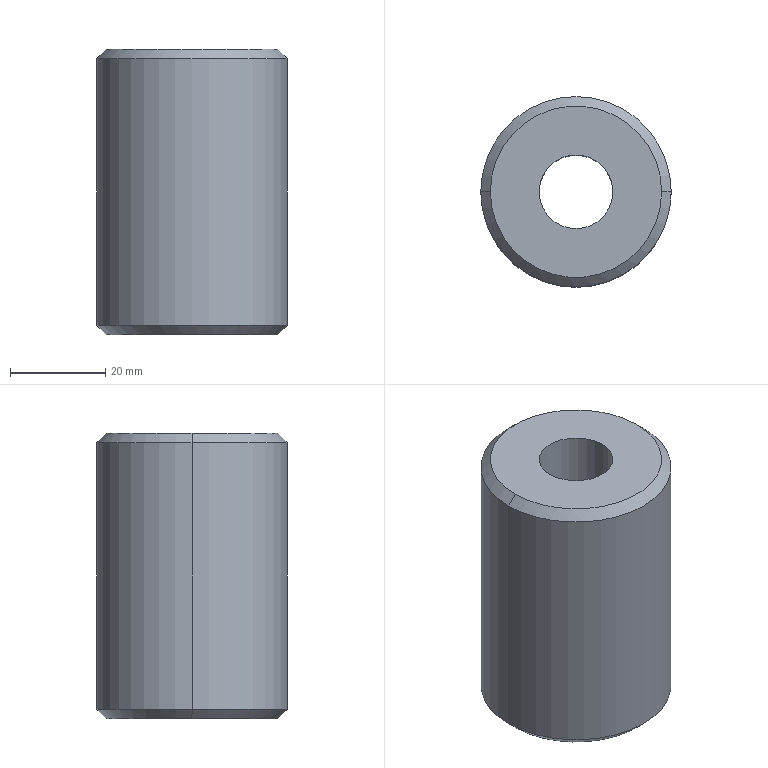Part | SolidWorks | features Chamfer 1, Extrusion 1, HoleWzd 1 | 1 solid | 10 faces | box 40 x 40 x 60 mm | volume 63591 mm3 | cylinder 4 | cone 4 | plane 2 | commonest cylinder face diameters 15.5 x2 40 x2
STEP:
#1=CARTESIAN_POINT('',(-7.75,0.,-30.));
#2=VERTEX_POINT('',#1);
#3=CARTESIAN_POINT('',(7.75,0.,-30.));
#4=VERTEX_POINT('',#3);
#5=CARTESIAN_POINT('',(0.,0.,-30.));
#6=DIRECTION('',(0.,0.,1.));
#7=DIRECTION('',(1.,0.,0.));
#8=AXIS2_PLACEMENT_3D('',#5,#6,#7);
#9=CIRCLE('',#8,7.75);
#10=EDGE_CURVE('',#2,#4,#9,.T.);
#11=ORIENTED_EDGE('',*,*,#10,.F.);
#12=CARTESIAN_POINT('',(-7.75,0.,30.));
#13=VERTEX_POINT('',#12);
#14=CARTESIAN_POINT('',(-7.75,0.,30.));
#15=DIRECTION('',(0.,0.,1.));
#16=VECTOR('',#15,1000.);
#17=LINE('',#14,#16);
#18=EDGE_CURVE('',#2,#13,#17,.T.);
#19=ORIENTED_EDGE('',*,*,#18,.T.);
#20=CARTESIAN_POINT('',(7.75,0.,30.));
#21=VERTEX_POINT('',#20);
#22=CARTESIAN_POINT('',(0.,0.,30.));
#23=DIRECTION('',(0.,0.,1.));
#24=DIRECTION('',(1.,0.,0.));
#25=AXIS2_PLACEMENT_3D('',#22,#23,#24);
#26=CIRCLE('',#25,7.75);
#27=EDGE_CURVE('',#13,#21,#26,.T.);
#28=ORIENTED_EDGE('',*,*,#27,.T.);
#29=CARTESIAN_POINT('',(7.75,0.,30.));
#30=DIRECTION('',(0.,0.,1.));
#31=VECTOR('',#30,1000.);
#32=LINE('',#29,#31);
#33=EDGE_CURVE('',#4,#21,#32,.T.);
#34=ORIENTED_EDGE('',*,*,#33,.F.);
#35=EDGE_LOOP('',(#11,#19,#28,#34));
#36=FACE_OUTER_BOUND('',#35,.T.);
#37=CARTESIAN_POINT('',(0.,0.,30.));
#38=DIRECTION('',(0.,0.,1.));
#39=DIRECTION('',(1.,0.,0.));
#40=AXIS2_PLACEMENT_3D('',#37,#38,#39);
#41=CYLINDRICAL_SURFACE('',#40,7.75);
#42=ADVANCED_FACE('',(#36),#41,.F.);
#43=CARTESIAN_POINT('',(18.,0.,30.));
#44=VERTEX_POINT('',#43);
#45=CARTESIAN_POINT('',(-18.,0.,30.));
#46=VERTEX_POINT('',#45);
#47=CARTESIAN_POINT('',(0.,0.,30.));
#48=DIRECTION('',(0.,0.,1.));
#49=DIRECTION('',(1.,0.,0.));
#50=AXIS2_PLACEMENT_3D('',#47,#48,#49);
#51=CIRCLE('',#50,18.);
#52=EDGE_CURVE('',#44,#46,#51,.T.);
#53=ORIENTED_EDGE('',*,*,#52,.F.);
#54=CARTESIAN_POINT('',(20.,0.,28.));
#55=VERTEX_POINT('',#54);
#56=CARTESIAN_POINT('',(18.,0.,30.));
#57=DIRECTION('',(0.7071,0.,-0.7071));
#58=VECTOR('',#57,1000.);
#59=LINE('',#56,#58);
#60=EDGE_CURVE('',#44,#55,#59,.T.);
#61=ORIENTED_EDGE('',*,*,#60,.T.);
#62=CARTESIAN_POINT('',(-20.,0.,28.));
#63=VERTEX_POINT('',#62);
#64=CARTESIAN_POINT('',(0.,0.,28.));
#65=DIRECTION('',(0.,0.,-1.));
#66=DIRECTION('',(1.,0.,0.));
#67=AXIS2_PLACEMENT_3D('',#64,#65,#66);
#68=CIRCLE('',#67,20.);
#69=EDGE_CURVE('',#63,#55,#68,.T.);
#70=ORIENTED_EDGE('',*,*,#69,.F.);
#71=CARTESIAN_POINT('',(-18.,0.,30.));
#72=DIRECTION('',(-0.7071,0.,-0.7071));
#73=VECTOR('',#72,1000.);
#74=LINE('',#71,#73);
#75=EDGE_CURVE('',#46,#63,#74,.T.);
#76=ORIENTED_EDGE('',*,*,#75,.F.);
#77=EDGE_LOOP('',(#53,#61,#70,#76));
#78=FACE_OUTER_BOUND('',#77,.T.);
#79=CARTESIAN_POINT('',(0.,0.,30.));
#80=DIRECTION('',(0.,0.,-1.));
#81=DIRECTION('',(-1.,0.,0.));
#82=AXIS2_PLACEMENT_3D('',#79,#80,#81);
#83=CONICAL_SURFACE('',#82,18.,0.7854);
#84=ADVANCED_FACE('',(#78),#83,.T.);
#85=CARTESIAN_POINT('',(-18.,0.,-30.));
#86=VERTEX_POINT('',#85);
#87=CARTESIAN_POINT('',(18.,0.,-30.));
#88=VERTEX_POINT('',#87);
#89=CARTESIAN_POINT('',(0.,0.,-30.));
#90=DIRECTION('',(0.,0.,-1.));
#91=DIRECTION('',(1.,0.,0.));
#92=AXIS2_PLACEMENT_3D('',#89,#90,#91);
#93=CIRCLE('',#92,18.);
#94=EDGE_CURVE('',#86,#88,#93,.T.);
#95=ORIENTED_EDGE('',*,*,#94,.F.);
#96=CARTESIAN_POINT('',(-20.,0.,-28.));
#97=VERTEX_POINT('',#96);
#98=CARTESIAN_POINT('',(-20.,0.,-28.));
#99=DIRECTION('',(-0.7071,0.,0.7071));
#100=VECTOR('',#99,1000.);
#101=LINE('',#98,#100);
#102=EDGE_CURVE('',#86,#97,#101,.T.);
#103=ORIENTED_EDGE('',*,*,#102,.T.);
#104=CARTESIAN_POINT('',(20.,0.,-28.));
#105=VERTEX_POINT('',#104);
#106=CARTESIAN_POINT('',(0.,0.,-28.));
#107=DIRECTION('',(0.,0.,1.));
#108=DIRECTION('',(1.,0.,0.));
#109=AXIS2_PLACEMENT_3D('',#106,#107,#108);
#110=CIRCLE('',#109,20.);
#111=EDGE_CURVE('',#105,#97,#110,.T.);
#112=ORIENTED_EDGE('',*,*,#111,.F.);
#113=CARTESIAN_POINT('',(20.,0.,-28.));
#114=DIRECTION('',(0.7071,0.,0.7071));
#115=VECTOR('',#114,1000.);
#116=LINE('',#113,#115);
#117=EDGE_CURVE('',#88,#105,#116,.T.);
#118=ORIENTED_EDGE('',*,*,#117,.F.);
#119=EDGE_LOOP('',(#95,#103,#112,#118));
#120=FACE_OUTER_BOUND('',#119,.T.);
#121=CARTESIAN_POINT('',(0.,0.,-28.));
#122=DIRECTION('',(0.,0.,1.));
#123=DIRECTION('',(1.,0.,0.));
#124=AXIS2_PLACEMENT_3D('',#121,#122,#123);
#125=CONICAL_SURFACE('',#124,20.,0.7854);
#126=ADVANCED_FACE('',(#120),#125,.T.);
#127=ORIENTED_EDGE('',*,*,#69,.T.);
#128=CARTESIAN_POINT('',(20.,0.,30.));
#129=DIRECTION('',(0.,0.,-1.));
#130=VECTOR('',#129,1000.);
#131=LINE('',#128,#130);
#132=EDGE_CURVE('',#55,#105,#131,.T.);
#133=ORIENTED_EDGE('',*,*,#132,.T.);
#134=ORIENTED_EDGE('',*,*,#111,.T.);
#135=CARTESIAN_POINT('',(-20.,0.,30.));
#136=DIRECTION('',(0.,0.,-1.));
#137=VECTOR('',#136,1000.);
#138=LINE('',#135,#137);
#139=EDGE_CURVE('',#63,#97,#138,.T.);
#140=ORIENTED_EDGE('',*,*,#139,.F.);
#141=EDGE_LOOP('',(#127,#133,#134,#140));
#142=FACE_OUTER_BOUND('',#141,.T.);
#143=CARTESIAN_POINT('',(0.,0.,30.));
#144=DIRECTION('',(0.,0.,-1.));
#145=DIRECTION('',(-1.,0.,0.));
#146=AXIS2_PLACEMENT_3D('',#143,#144,#145);
#147=CYLINDRICAL_SURFACE('',#146,20.);
#148=ADVANCED_FACE('',(#142),#147,.T.);
#149=ORIENTED_EDGE('',*,*,#132,.F.);
#150=CARTESIAN_POINT('',(0.,0.,28.));
#151=DIRECTION('',(0.,0.,-1.));
#152=DIRECTION('',(1.,0.,0.));
#153=AXIS2_PLACEMENT_3D('',#150,#151,#152);
#154=CIRCLE('',#153,20.);
#155=EDGE_CURVE('',#55,#63,#154,.T.);
#156=ORIENTED_EDGE('',*,*,#155,.T.);
#157=ORIENTED_EDGE('',*,*,#139,.T.);
#158=CARTESIAN_POINT('',(0.,0.,-28.));
#159=DIRECTION('',(0.,0.,1.));
#160=DIRECTION('',(1.,0.,0.));
#161=AXIS2_PLACEMENT_3D('',#158,#159,#160);
#162=CIRCLE('',#161,20.);
#163=EDGE_CURVE('',#97,#105,#162,.T.);
#164=ORIENTED_EDGE('',*,*,#163,.T.);
#165=EDGE_LOOP('',(#149,#156,#157,#164));
#166=FACE_OUTER_BOUND('',#165,.T.);
#167=CARTESIAN_POINT('',(0.,0.,30.));
#168=DIRECTION('',(0.,0.,-1.));
#169=DIRECTION('',(-1.,0.,0.));
#170=AXIS2_PLACEMENT_3D('',#167,#168,#169);
#171=CYLINDRICAL_SURFACE('',#170,20.);
#172=ADVANCED_FACE('',(#166),#171,.T.);
#173=CARTESIAN_POINT('',(0.,0.,30.));
#174=DIRECTION('',(0.,0.,1.));
#175=DIRECTION('',(1.,0.,0.));
#176=AXIS2_PLACEMENT_3D('',#173,#174,#175);
#177=CIRCLE('',#176,7.75);
#178=EDGE_CURVE('',#21,#13,#177,.T.);
#179=ORIENTED_EDGE('',*,*,#178,.F.);
#180=ORIENTED_EDGE('',*,*,#27,.F.);
#181=EDGE_LOOP('',(#179,#180));
#182=FACE_BOUND('',#181,.T.);
#183=CARTESIAN_POINT('',(0.,0.,30.));
#184=DIRECTION('',(0.,0.,1.));
#185=DIRECTION('',(1.,0.,0.));
#186=AXIS2_PLACEMENT_3D('',#183,#184,#185);
#187=CIRCLE('',#186,18.);
#188=EDGE_CURVE('',#46,#44,#187,.T.);
#189=ORIENTED_EDGE('',*,*,#188,.T.);
#190=ORIENTED_EDGE('',*,*,#52,.T.);
#191=EDGE_LOOP('',(#189,#190));
#192=FACE_OUTER_BOUND('',#191,.T.);
#193=CARTESIAN_POINT('',(0.,0.,30.));
#194=DIRECTION('',(0.,0.,1.));
#195=DIRECTION('',(1.,0.,0.));
#196=AXIS2_PLACEMENT_3D('',#193,#194,#195);
#197=PLANE('',#196);
#198=ADVANCED_FACE('',(#182,#192),#197,.T.);
#199=CARTESIAN_POINT('',(0.,0.,-30.));
#200=DIRECTION('',(0.,0.,1.));
#201=DIRECTION('',(1.,0.,0.));
#202=AXIS2_PLACEMENT_3D('',#199,#200,#201);
#203=CIRCLE('',#202,7.75);
#204=EDGE_CURVE('',#4,#2,#203,.T.);
#205=ORIENTED_EDGE('',*,*,#204,.T.);
#206=ORIENTED_EDGE('',*,*,#10,.T.);
#207=EDGE_LOOP('',(#205,#206));
#208=FACE_BOUND('',#207,.T.);
#209=CARTESIAN_POINT('',(0.,0.,-30.));
#210=DIRECTION('',(0.,0.,-1.));
#211=DIRECTION('',(1.,0.,0.));
#212=AXIS2_PLACEMENT_3D('',#209,#210,#211);
#213=CIRCLE('',#212,18.);
#214=EDGE_CURVE('',#88,#86,#213,.T.);
#215=ORIENTED_EDGE('',*,*,#214,.T.);
#216=ORIENTED_EDGE('',*,*,#94,.T.);
#217=EDGE_LOOP('',(#215,#216));
#218=FACE_OUTER_BOUND('',#217,.T.);
#219=CARTESIAN_POINT('',(0.,0.,-30.));
#220=DIRECTION('',(0.,0.,1.));
#221=DIRECTION('',(1.,0.,0.));
#222=AXIS2_PLACEMENT_3D('',#219,#220,#221);
#223=PLANE('',#222);
#224=ADVANCED_FACE('',(#208,#218),#223,.F.);
#225=ORIENTED_EDGE('',*,*,#102,.F.);
#226=ORIENTED_EDGE('',*,*,#214,.F.);
#227=ORIENTED_EDGE('',*,*,#117,.T.);
#228=ORIENTED_EDGE('',*,*,#163,.F.);
#229=EDGE_LOOP('',(#225,#226,#227,#228));
#230=FACE_OUTER_BOUND('',#229,.T.);
#231=CARTESIAN_POINT('',(0.,0.,-28.));
#232=DIRECTION('',(0.,0.,1.));
#233=DIRECTION('',(1.,0.,0.));
#234=AXIS2_PLACEMENT_3D('',#231,#232,#233);
#235=CONICAL_SURFACE('',#234,20.,0.7854);
#236=ADVANCED_FACE('',(#230),#235,.T.);
#237=ORIENTED_EDGE('',*,*,#60,.F.);
#238=ORIENTED_EDGE('',*,*,#188,.F.);
#239=ORIENTED_EDGE('',*,*,#75,.T.);
#240=ORIENTED_EDGE('',*,*,#155,.F.);
#241=EDGE_LOOP('',(#237,#238,#239,#240));
#242=FACE_OUTER_BOUND('',#241,.T.);
#243=CARTESIAN_POINT('',(0.,0.,30.));
#244=DIRECTION('',(0.,0.,-1.));
#245=DIRECTION('',(-1.,0.,0.));
#246=AXIS2_PLACEMENT_3D('',#243,#244,#245);
#247=CONICAL_SURFACE('',#246,18.,0.7854);
#248=ADVANCED_FACE('',(#242),#247,.T.);
#249=ORIENTED_EDGE('',*,*,#18,.F.);
#250=ORIENTED_EDGE('',*,*,#204,.F.);
#251=ORIENTED_EDGE('',*,*,#33,.T.);
#252=ORIENTED_EDGE('',*,*,#178,.T.);
#253=EDGE_LOOP('',(#249,#250,#251,#252));
#254=FACE_OUTER_BOUND('',#253,.T.);
#255=CARTESIAN_POINT('',(0.,0.,30.));
#256=DIRECTION('',(0.,0.,1.));
#257=DIRECTION('',(1.,0.,0.));
#258=AXIS2_PLACEMENT_3D('',#255,#256,#257);
#259=CYLINDRICAL_SURFACE('',#258,7.75);
#260=ADVANCED_FACE('',(#254),#259,.F.);
#261=CLOSED_SHELL('',(#42,#84,#126,#148,#172,#198,#224,#236,#248,#260));
#262=MANIFOLD_SOLID_BREP('',#261);
#263=CARTESIAN_POINT('',(0.,0.,0.));
#264=DIRECTION('',(0.,0.,1.));
#265=DIRECTION('',(1.,0.,0.));
#266=AXIS2_PLACEMENT_3D('',#263,#264,#265);
#267=(LENGTH_UNIT()NAMED_UNIT(*)SI_UNIT(.MILLI.,.METRE.));
#268=UNCERTAINTY_MEASURE_WITH_UNIT(LENGTH_MEASURE(0.00001),#267,'','');
#269=(NAMED_UNIT(*)PLANE_ANGLE_UNIT()SI_UNIT($,.RADIAN.));
#270=(NAMED_UNIT(*)SI_UNIT($,.STERADIAN.)SOLID_ANGLE_UNIT());
#271=(GEOMETRIC_REPRESENTATION_CONTEXT(3)GLOBAL_UNCERTAINTY_ASSIGNED_CONTEXT((#268))GLOBAL_UNIT_ASSIGNED_CONTEXT((#267,#269,#270))REPRESENTATION_CONTEXT('',''));
#272=ADVANCED_BREP_SHAPE_REPRESENTATION('',(#262,#266),#271);